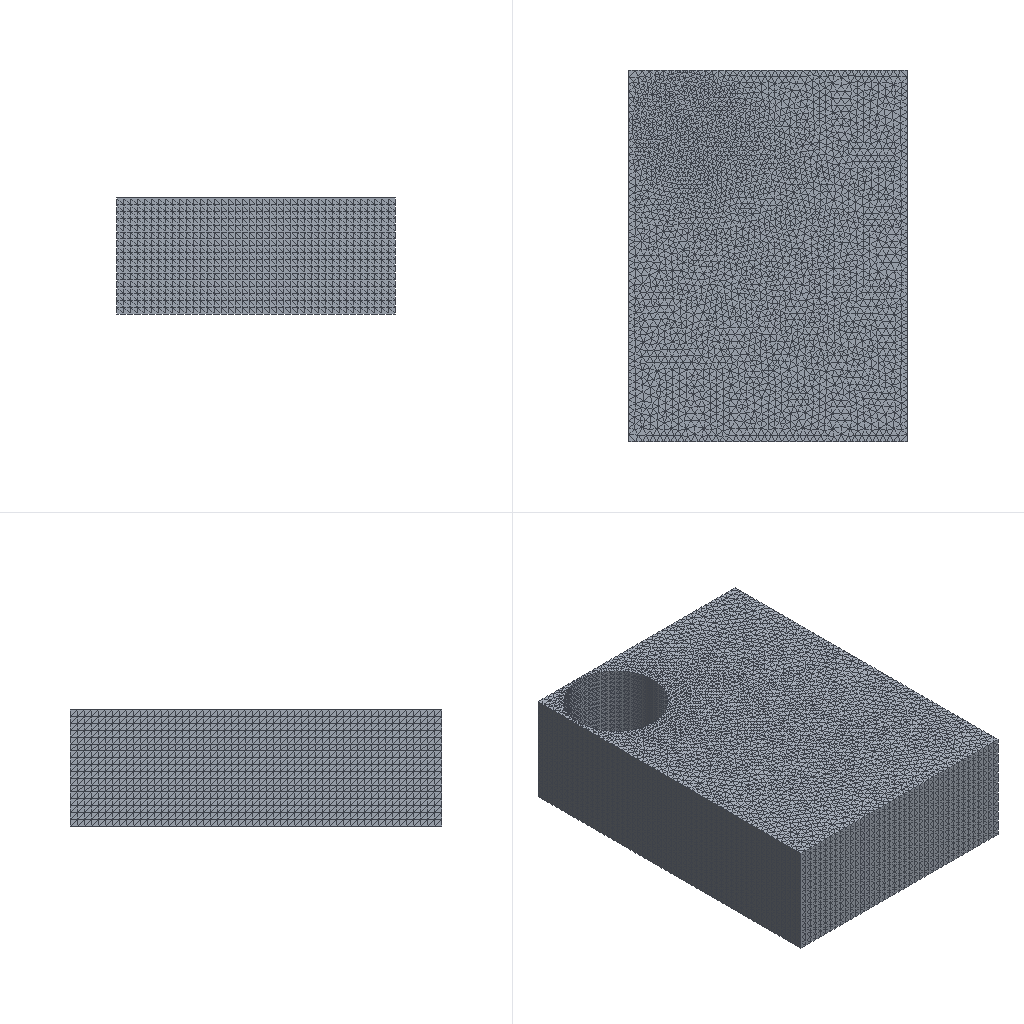Simulation study | abaqus
Set-up summary:
category,name,step,type,value,unit,region
solver,abaqus
solver,version,,,Abaqus/Explicit 2020
units,not stated in the deck,,not stated
analysis,deck,,transient,transient
load_step,Step-1,Step-1,transient
load_step,requested,,,1
mesh,nodes,,,42365
mesh,elements,,,210107
element_type,C3D4,,solid,201965
element_type,R3D3,,rigid,8142
load,load commands in deck,,count,3
bc,support commands in deck,,count,7
material,MATERIAL-1,,in results
check,setup vs results,,match,"per instance, exact: element labels, types and connectivity; labels of the nodes the elements use; coordinates of those nodes at SINGLE_PRECISION in 2 of 2 instance(s)"
Abaqus input file, long lists of numbers shortened:
*Heading
** Job name: Job-1 Model name: Model-1
** Generated by: Abaqus/CAE 2020
*Preprint, echo=NO, model=NO, history=NO, contact=NO
**
** PARTS
**
*Part, name=daojiu
*Node
      1,           3.,           0.,         -35.
      2,           3.,           0.,         -20.
** (4065 more lines like these left out)
*Element, type=R3D3
 1,    1,  644, 2335
 2, 2335, 2342,    1
** (8140 more lines like these left out)
*Node
   4068, 4.36618125e-15, -3.55271368e-15,  -59.35
*Nset, nset=daojiu-RefPt_, internal
4068,
*Elset, elset=daojiu, generate
    1,  8142,     1
*End Part
**
*Part, name=gongjian
*Node
      1,         -60.,          90.,           0.
      2,          60.,          90.,           0.
** (38295 more lines like these left out)
*Element, type=C3D4
     1,  9579,  9580,  9581,  9582
     2,  9583,  9584,  9582,  9579
** (201963 more lines like these left out)
*Nset, nset=Set-4, generate
     1,  38297,      1
*Elset, elset=Set-4, generate
      1,  201965,       1
** Section: Section-1
*Solid Section, elset=Set-4, material=Material-1
,
*End Part
**
**
** ASSEMBLY
**
*Assembly, name=Assembly
**
*Instance, name=daojiu-1, part=daojiu
        -36.,         66.5,    70.35
*End Instance
**
*Instance, name=gongjian-1, part=gongjian
*End Instance
**
*Nset, nset=Set-1, instance=gongjian-1
    1,    2,    3,    4,   13,   14,   15,   16,   17,   18,   19,   20,   21,   22,   23,   24
   25,   26,   27,   28,   29,   30,   31,   32,   33,   34,   35,   36,   37,   38,   39,   40
** (137 more lines like these left out)
*Elset, elset=Set-1, instance=gongjian-1
    379,    905,   1065,   1568,   1606,   1821,   1911,   2725,   3323,   3403,   3615,   3777,   4043,   4776,   6390,   6456
   7045,   7619,   7762,   7857,   8162,   8186,   8534,   8776,   8889,   8980,   9236,   9293,   9444,   9484,   9502,  10297
** (263 more lines like these left out)
*Nset, nset=Set-2, instance=daojiu-1
 4068,
*Nset, nset=Set-4, instance=daojiu-1
 4068,
*Nset, nset=s_Set-3, instance=gongjian-1, generate
     1,  38297,      1
*Elset, elset=s_Set-3, instance=gongjian-1, generate
      1,  201965,       1
*Elset, elset=_m_Surf-1_SPOS, internal, instance=daojiu-1, generate
 3148,  3233,     1
*Surface, type=ELEMENT, name=m_Surf-1
_m_Surf-1_SPOS, SPOS
*Elset, elset=_m_Surf-2_SPOS, internal, instance=daojiu-1, generate
 2588,  2673,     1
*Surface, type=ELEMENT, name=m_Surf-2
_m_Surf-2_SPOS, SPOS
*Elset, elset=_m_Surf-3_SPOS, internal, instance=daojiu-1, generate
 2028,  2113,     1
*Surface, type=ELEMENT, name=m_Surf-3
_m_Surf-3_SPOS, SPOS
*Elset, elset=_m_Surf-4_SPOS, internal, instance=daojiu-1, generate
 3760,  3845,     1
*Surface, type=ELEMENT, name=m_Surf-4
_m_Surf-4_SPOS, SPOS
*Elset, elset=_m_Surf-5_SPOS, internal, instance=daojiu-1
  901,  902,  903,  904,  905,  906,  907,  908,  909,  910,  911,  912,  913,  914,  915,  916
  917,  918,  919,  920,  921,  922,  923,  924,  925,  926,  927,  928,  929,  930,  931,  932
** (8 more lines like these left out)
*Surface, type=ELEMENT, name=m_Surf-5
_m_Surf-5_SPOS, SPOS
*Elset, elset=_m_Surf-6_SPOS, internal, instance=daojiu-1
  633,  634,  635,  636,  637,  638,  639,  640,  641,  642,  643,  644,  645,  646,  647,  648
  649,  650,  651,  652,  653,  654,  655,  656,  657,  658,  659,  660,  661,  662,  663,  664
** (8 more lines like these left out)
*Surface, type=ELEMENT, name=m_Surf-6
_m_Surf-6_SPOS, SPOS
*Elset, elset=_m_Surf-7_SPOS, internal, instance=daojiu-1
  365,  366,  367,  368,  369,  370,  371,  372,  373,  374,  375,  376,  377,  378,  379,  380
  381,  382,  383,  384,  385,  386,  387,  388,  389,  390,  391,  392,  393,  394,  395,  396
** (8 more lines like these left out)
*Surface, type=ELEMENT, name=m_Surf-7
_m_Surf-7_SPOS, SPOS
*Elset, elset=_m_Surf-8_SPOS, internal, instance=daojiu-1
   97,   98,   99,  100,  101,  102,  103,  104,  105,  106,  107,  108,  109,  110,  111,  112
  113,  114,  115,  116,  117,  118,  119,  120,  121,  122,  123,  124,  125,  126,  127,  128
** (8 more lines like these left out)
*Surface, type=ELEMENT, name=m_Surf-8
_m_Surf-8_SPOS, SPOS
*Rigid Body, ref node=daojiu-1.daojiu-RefPt_, elset=daojiu-1.daojiu
*End Assembly
*Amplitude, name=Amp-1, definition=PERIODIC
1,           1256.,              0.,              0.
             1.,              0.
**
** MATERIALS
**
*Material, name=Material-1
*Damage Initiation, criterion=JOHNSON COOK
 -0.09,  0.25,  -0.5, 0.014,  3.87, 1650.,   25.,    1.
*Damage Evolution, type=DISPLACEMENT
 1e-05,
*Density
 4.4e-09,
*Elastic
108000., 0.33
*Plastic, hardening=JOHNSON COOK
860., 683., 0.47,   1.,1650.,  25.
*Rate Dependent, type=JOHNSON COOK
 0.035,1.
**
** INTERACTION PROPERTIES
**
*Surface Interaction, name=IntProp-1
*Friction
 0.15,
*Surface Behavior, pressure-overclosure=HARD
** ----------------------------------------------------------------
**
** STEP: Step-1
**
*Step, name=Step-1, nlgeom=YES
*Dynamic, Explicit
, 0.1
*Bulk Viscosity
0.06, 1.2
** Mass Scaling: Semi-Automatic
**               Whole Model
*Fixed Mass Scaling, factor=5000.
**
** BOUNDARY CONDITIONS
**
** Name: BC-1 Type: 对称/反对称/完全固定
*Boundary
Set-1, ENCASTRE
** Name: [REDACTED]
*Boundary, amplitude=Amp-1
Set-4, 3, 3, -20.
** Name: [REDACTED] : Velocity/Angular velocity
*Boundary, type=VELOCITY
Set-2, 1, 1
Set-2, 2, 2, -1200.
Set-2, 4, 4
Set-2, 5, 5
Set-2, 6, 6, -400.
**
** INTERACTIONS
**
** Interaction: Int-9
*Contact, op=NEW
*Contact Inclusions, ALL EXTERIOR
*Contact Property Assignment
 ,  , IntProp-1
**
** OUTPUT REQUESTS
**
*Restart, write, number interval=1, time marks=NO
**
** FIELD OUTPUT: F-Output-1
**
*Output, field, number interval=50
*Node Output
A, CF, RF, RM, RT, U, V
*Element Output, directions=YES
E, EVF, LE, MISES, MISESMAX, PE, PEEQ, PEEQVAVG, PEVAVG, S, STATUS, SVAVG
*Contact Output
CDISP, CSTRESS
**
** HISTORY OUTPUT: H-Output-1
**
*Output, history, time interval=2e-06
*Node Output, nset=Set-2
RF1, RF2, RF3
*End Step
Results summary:
result,step,Step-1,partial,increments=9431 time=0.0831/0.1
result,analysis,,,transient
result,last_loadstep,,,1
result,primary field,,,U
result,reaction total,,FX,-35582.543,model units
result,reaction total,,FY,-33732.393,model units
result,reaction total,,FZ,-78262.925,model units